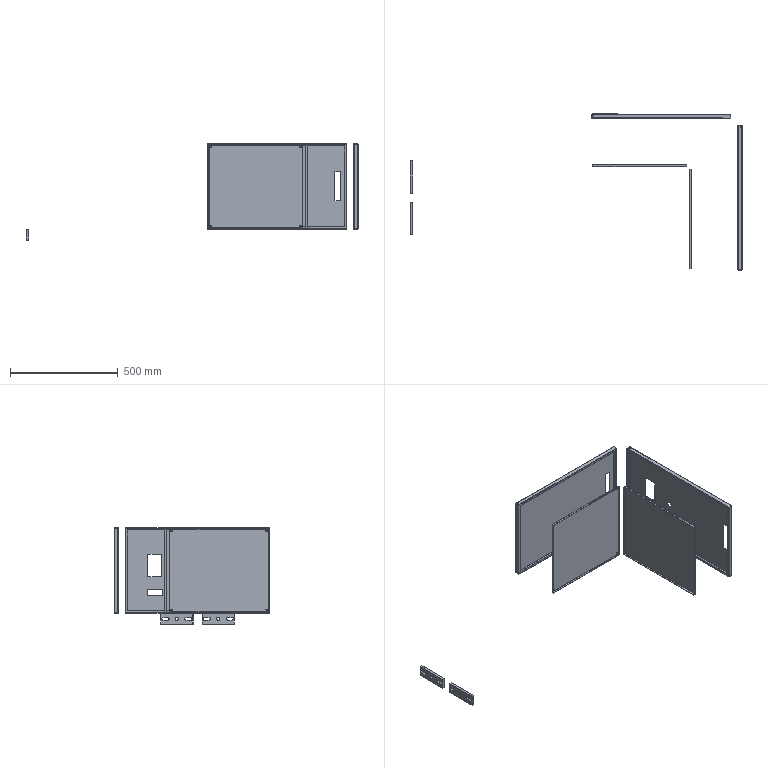Part | SolidWorks | 6 solids | 396 faces | box 1542 x 724.002 x 448 mm | volume 1639725 mm3 | plane 268 | cylinder 88 | cone 24 | spline 16 | commonest cylinder face diameters 0.4 x24 3.4 x24 7 x16 5.1 x8 11 x8 14 x4